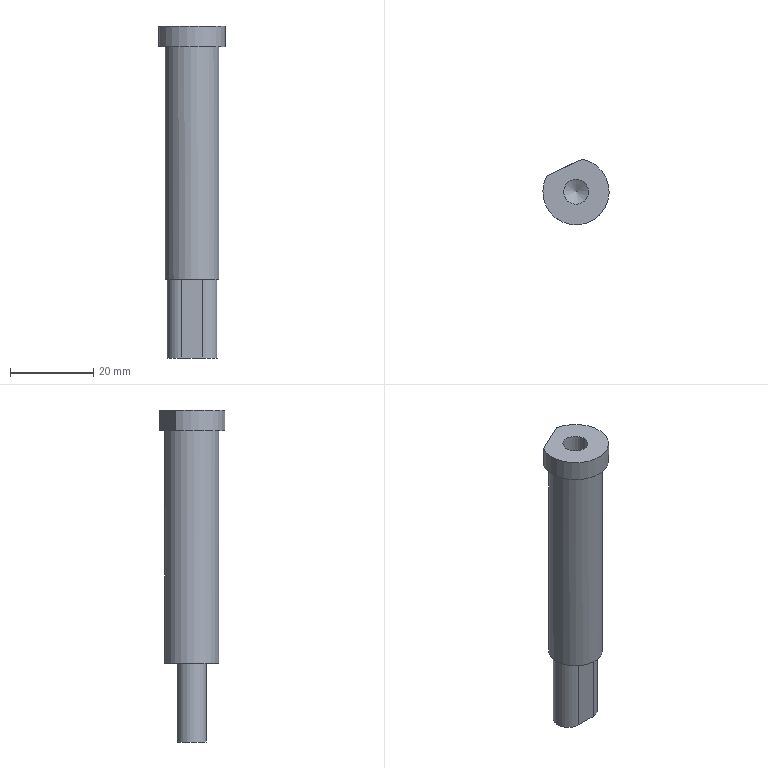Part | NX | features solid 2 | 1 solid | 13 faces | box 16 x 15.862 x 80 mm | volume 9434 mm3 | plane 7 | cylinder 5 | cone 1 | commonest cylinder face diameters 7.1 x2 6 x1 13 x1 16 x1
STEP:
#1=CARTESIAN_POINT('',(-654.921,-401.954,29.));
#2=VERTEX_POINT('',#1);
#3=CARTESIAN_POINT('',(-654.921,-408.454,29.));
#4=DIRECTION('',(0.,0.,1.));
#5=DIRECTION('',(0.,1.,0.));
#6=AXIS2_PLACEMENT_3D('',#3,#4,#5);
#7=CIRCLE('',#6,6.5);
#8=EDGE_CURVE('',#2,#2,#7,.T.);
#9=ORIENTED_EDGE('',*,*,#8,.F.);
#10=EDGE_LOOP('',(#9));
#11=FACE_BOUND('',#10,.T.);
#12=CARTESIAN_POINT('',(-657.421,-404.904,29.));
#13=VERTEX_POINT('',#12);
#14=CARTESIAN_POINT('',(-652.421,-404.904,29.));
#15=VERTEX_POINT('',#14);
#16=CARTESIAN_POINT('',(-654.921,-404.904,29.));
#17=DIRECTION('',(1.,0.,0.));
#18=VECTOR('',#17,1000.);
#19=LINE('',#16,#18);
#20=EDGE_CURVE('',#13,#15,#19,.T.);
#21=ORIENTED_EDGE('',*,*,#20,.F.);
#22=CARTESIAN_POINT('',(-657.421,-412.004,29.));
#23=VERTEX_POINT('',#22);
#24=CARTESIAN_POINT('',(-657.421,-408.454,29.));
#25=DIRECTION('',(0.,0.,1.));
#26=DIRECTION('',(0.,1.,0.));
#27=AXIS2_PLACEMENT_3D('',#24,#25,#26);
#28=CIRCLE('',#27,3.55);
#29=EDGE_CURVE('',#13,#23,#28,.T.);
#30=ORIENTED_EDGE('',*,*,#29,.T.);
#31=CARTESIAN_POINT('',(-652.421,-412.004,29.));
#32=VERTEX_POINT('',#31);
#33=CARTESIAN_POINT('',(-654.921,-412.004,29.));
#34=DIRECTION('',(1.,0.,0.));
#35=VECTOR('',#34,1000.);
#36=LINE('',#33,#35);
#37=EDGE_CURVE('',#23,#32,#36,.T.);
#38=ORIENTED_EDGE('',*,*,#37,.T.);
#39=CARTESIAN_POINT('',(-652.421,-408.454,29.));
#40=DIRECTION('',(0.,0.,1.));
#41=DIRECTION('',(0.,1.,0.));
#42=AXIS2_PLACEMENT_3D('',#39,#40,#41);
#43=CIRCLE('',#42,3.55);
#44=EDGE_CURVE('',#32,#15,#43,.T.);
#45=ORIENTED_EDGE('',*,*,#44,.T.);
#46=EDGE_LOOP('',(#21,#30,#38,#45));
#47=FACE_BOUND('',#46,.T.);
#48=CARTESIAN_POINT('',(-654.921,-408.454,29.));
#49=DIRECTION('',(0.,0.,1.));
#50=DIRECTION('',(0.,1.,0.));
#51=AXIS2_PLACEMENT_3D('',#48,#49,#50);
#52=PLANE('',#51);
#53=ADVANCED_FACE('',(#11,#47),#52,.F.);
#54=ORIENTED_EDGE('',*,*,#8,.T.);
#55=EDGE_LOOP('',(#54));
#56=FACE_BOUND('',#55,.T.);
#57=CARTESIAN_POINT('',(-657.668,-402.563,85.));
#58=VERTEX_POINT('',#57);
#59=CARTESIAN_POINT('',(-654.921,-408.454,85.));
#60=DIRECTION('',(0.,0.,1.));
#61=DIRECTION('',(0.,1.,0.));
#62=AXIS2_PLACEMENT_3D('',#59,#60,#61);
#63=CIRCLE('',#62,6.5);
#64=EDGE_CURVE('',#58,#58,#63,.T.);
#65=ORIENTED_EDGE('',*,*,#64,.F.);
#66=EDGE_LOOP('',(#65));
#67=FACE_BOUND('',#66,.T.);
#68=CARTESIAN_POINT('',(-654.921,-408.454,90.));
#69=DIRECTION('',(0.,0.,-1.));
#70=DIRECTION('',(0.,-1.,0.));
#71=AXIS2_PLACEMENT_3D('',#68,#69,#70);
#72=CYLINDRICAL_SURFACE('',#71,6.5);
#73=ADVANCED_FACE('',(#56,#67),#72,.T.);
#74=CARTESIAN_POINT('',(-661.894,-404.534,85.));
#75=VERTEX_POINT('',#74);
#76=CARTESIAN_POINT('',(-653.441,-400.592,85.));
#77=VERTEX_POINT('',#76);
#78=CARTESIAN_POINT('',(-654.921,-408.454,85.));
#79=DIRECTION('',(0.,0.,1.));
#80=DIRECTION('',(0.,1.,0.));
#81=AXIS2_PLACEMENT_3D('',#78,#79,#80);
#82=CIRCLE('',#81,8.);
#83=EDGE_CURVE('',#75,#77,#82,.T.);
#84=ORIENTED_EDGE('',*,*,#83,.F.);
#85=CARTESIAN_POINT('',(-653.441,-400.592,85.));
#86=DIRECTION('',(0.9063,0.4226,0.));
#87=VECTOR('',#86,1000.);
#88=LINE('',#85,#87);
#89=EDGE_CURVE('',#75,#58,#88,.T.);
#90=ORIENTED_EDGE('',*,*,#89,.T.);
#91=ORIENTED_EDGE('',*,*,#64,.T.);
#92=CARTESIAN_POINT('',(-653.441,-400.592,85.));
#93=DIRECTION('',(0.9063,0.4226,0.));
#94=VECTOR('',#93,1000.);
#95=LINE('',#92,#94);
#96=EDGE_CURVE('',#58,#77,#95,.T.);
#97=ORIENTED_EDGE('',*,*,#96,.T.);
#98=EDGE_LOOP('',(#84,#90,#91,#97));
#99=FACE_BOUND('',#98,.T.);
#100=CARTESIAN_POINT('',(-654.921,-408.454,85.));
#101=DIRECTION('',(0.,0.,1.));
#102=DIRECTION('',(0.,1.,0.));
#103=AXIS2_PLACEMENT_3D('',#100,#101,#102);
#104=PLANE('',#103);
#105=ADVANCED_FACE('',(#99),#104,.F.);
#106=CARTESIAN_POINT('',(-653.441,-400.592,90.));
#107=VERTEX_POINT('',#106);
#108=CARTESIAN_POINT('',(-653.441,-400.592,-87.));
#109=DIRECTION('',(0.,0.,-1.));
#110=VECTOR('',#109,1000.);
#111=LINE('',#108,#110);
#112=EDGE_CURVE('',#107,#77,#111,.T.);
#113=ORIENTED_EDGE('',*,*,#112,.F.);
#114=CARTESIAN_POINT('',(-661.894,-404.534,90.));
#115=VERTEX_POINT('',#114);
#116=CARTESIAN_POINT('',(-654.921,-408.454,90.));
#117=DIRECTION('',(0.,0.,1.));
#118=DIRECTION('',(0.,1.,0.));
#119=AXIS2_PLACEMENT_3D('',#116,#117,#118);
#120=CIRCLE('',#119,8.);
#121=EDGE_CURVE('',#115,#107,#120,.T.);
#122=ORIENTED_EDGE('',*,*,#121,.F.);
#123=CARTESIAN_POINT('',(-661.894,-404.534,-87.));
#124=DIRECTION('',(0.,0.,-1.));
#125=VECTOR('',#124,1000.);
#126=LINE('',#123,#125);
#127=EDGE_CURVE('',#75,#115,#126,.F.);
#128=ORIENTED_EDGE('',*,*,#127,.F.);
#129=ORIENTED_EDGE('',*,*,#83,.T.);
#130=EDGE_LOOP('',(#113,#122,#128,#129));
#131=FACE_BOUND('',#130,.T.);
#132=CARTESIAN_POINT('',(-654.921,-408.454,85.));
#133=DIRECTION('',(0.,0.,1.));
#134=DIRECTION('',(0.,1.,0.));
#135=AXIS2_PLACEMENT_3D('',#132,#133,#134);
#136=CYLINDRICAL_SURFACE('',#135,8.);
#137=ADVANCED_FACE('',(#131),#136,.T.);
#138=CARTESIAN_POINT('',(-654.921,-411.454,90.));
#139=VERTEX_POINT('',#138);
#140=CARTESIAN_POINT('',(-654.921,-408.454,90.));
#141=DIRECTION('',(0.,0.,-1.));
#142=DIRECTION('',(0.,-1.,0.));
#143=AXIS2_PLACEMENT_3D('',#140,#141,#142);
#144=CIRCLE('',#143,3.);
#145=EDGE_CURVE('',#139,#139,#144,.T.);
#146=ORIENTED_EDGE('',*,*,#145,.T.);
#147=EDGE_LOOP('',(#146));
#148=FACE_BOUND('',#147,.T.);
#149=CARTESIAN_POINT('',(-653.441,-400.592,90.));
#150=DIRECTION('',(0.9063,0.4226,0.));
#151=VECTOR('',#150,1000.);
#152=LINE('',#149,#151);
#153=EDGE_CURVE('',#115,#107,#152,.T.);
#154=ORIENTED_EDGE('',*,*,#153,.F.);
#155=ORIENTED_EDGE('',*,*,#121,.T.);
#156=EDGE_LOOP('',(#154,#155));
#157=FACE_BOUND('',#156,.T.);
#158=CARTESIAN_POINT('',(-654.921,-408.454,90.));
#159=DIRECTION('',(0.,0.,1.));
#160=DIRECTION('',(0.,1.,0.));
#161=AXIS2_PLACEMENT_3D('',#158,#159,#160);
#162=PLANE('',#161);
#163=ADVANCED_FACE('',(#148,#157),#162,.T.);
#164=ORIENTED_EDGE('',*,*,#127,.T.);
#165=ORIENTED_EDGE('',*,*,#153,.T.);
#166=ORIENTED_EDGE('',*,*,#112,.T.);
#167=ORIENTED_EDGE('',*,*,#96,.F.);
#168=ORIENTED_EDGE('',*,*,#89,.F.);
#169=EDGE_LOOP('',(#164,#165,#166,#167,#168));
#170=FACE_BOUND('',#169,.T.);
#171=CARTESIAN_POINT('',(-653.441,-400.592,-87.));
#172=DIRECTION('',(0.4226,-0.9063,0.));
#173=DIRECTION('',(0.,0.,-1.));
#174=AXIS2_PLACEMENT_3D('',#171,#172,#173);
#175=PLANE('',#174);
#176=ADVANCED_FACE('',(#170),#175,.F.);
#177=CARTESIAN_POINT('',(-657.421,-404.904,10.));
#178=VERTEX_POINT('',#177);
#179=CARTESIAN_POINT('',(-657.421,-404.904,10.));
#180=DIRECTION('',(0.,0.,1.));
#181=VECTOR('',#180,1000.);
#182=LINE('',#179,#181);
#183=EDGE_CURVE('',#178,#13,#182,.T.);
#184=ORIENTED_EDGE('',*,*,#183,.T.);
#185=ORIENTED_EDGE('',*,*,#20,.T.);
#186=CARTESIAN_POINT('',(-652.421,-404.904,10.));
#187=VERTEX_POINT('',#186);
#188=CARTESIAN_POINT('',(-652.421,-404.904,10.));
#189=DIRECTION('',(0.,0.,1.));
#190=VECTOR('',#189,1000.);
#191=LINE('',#188,#190);
#192=EDGE_CURVE('',#187,#15,#191,.T.);
#193=ORIENTED_EDGE('',*,*,#192,.F.);
#194=CARTESIAN_POINT('',(-657.421,-404.904,10.));
#195=DIRECTION('',(1.,0.,0.));
#196=VECTOR('',#195,1000.);
#197=LINE('',#194,#196);
#198=EDGE_CURVE('',#178,#187,#197,.T.);
#199=ORIENTED_EDGE('',*,*,#198,.F.);
#200=EDGE_LOOP('',(#184,#185,#193,#199));
#201=FACE_BOUND('',#200,.T.);
#202=CARTESIAN_POINT('',(-657.421,-404.904,10.));
#203=DIRECTION('',(0.,-1.,0.));
#204=DIRECTION('',(0.,0.,1.));
#205=AXIS2_PLACEMENT_3D('',#202,#203,#204);
#206=PLANE('',#205);
#207=ADVANCED_FACE('',(#201),#206,.F.);
#208=ORIENTED_EDGE('',*,*,#44,.F.);
#209=CARTESIAN_POINT('',(-652.421,-412.004,10.));
#210=VERTEX_POINT('',#209);
#211=CARTESIAN_POINT('',(-652.421,-412.004,10.));
#212=DIRECTION('',(0.,0.,1.));
#213=VECTOR('',#212,1000.);
#214=LINE('',#211,#213);
#215=EDGE_CURVE('',#210,#32,#214,.T.);
#216=ORIENTED_EDGE('',*,*,#215,.F.);
#217=CARTESIAN_POINT('',(-652.421,-408.454,10.));
#218=DIRECTION('',(0.,0.,1.));
#219=DIRECTION('',(0.,1.,0.));
#220=AXIS2_PLACEMENT_3D('',#217,#218,#219);
#221=CIRCLE('',#220,3.55);
#222=EDGE_CURVE('',#210,#187,#221,.T.);
#223=ORIENTED_EDGE('',*,*,#222,.T.);
#224=ORIENTED_EDGE('',*,*,#192,.T.);
#225=EDGE_LOOP('',(#208,#216,#223,#224));
#226=FACE_BOUND('',#225,.T.);
#227=CARTESIAN_POINT('',(-652.421,-408.454,10.));
#228=DIRECTION('',(0.,0.,1.));
#229=DIRECTION('',(0.,1.,0.));
#230=AXIS2_PLACEMENT_3D('',#227,#228,#229);
#231=CYLINDRICAL_SURFACE('',#230,3.55);
#232=ADVANCED_FACE('',(#226),#231,.T.);
#233=ORIENTED_EDGE('',*,*,#37,.F.);
#234=CARTESIAN_POINT('',(-657.421,-412.004,10.));
#235=VERTEX_POINT('',#234);
#236=CARTESIAN_POINT('',(-657.421,-412.004,10.));
#237=DIRECTION('',(0.,0.,1.));
#238=VECTOR('',#237,1000.);
#239=LINE('',#236,#238);
#240=EDGE_CURVE('',#235,#23,#239,.T.);
#241=ORIENTED_EDGE('',*,*,#240,.F.);
#242=CARTESIAN_POINT('',(-657.421,-412.004,10.));
#243=DIRECTION('',(1.,0.,0.));
#244=VECTOR('',#243,1000.);
#245=LINE('',#242,#244);
#246=EDGE_CURVE('',#235,#210,#245,.T.);
#247=ORIENTED_EDGE('',*,*,#246,.T.);
#248=ORIENTED_EDGE('',*,*,#215,.T.);
#249=EDGE_LOOP('',(#233,#241,#247,#248));
#250=FACE_BOUND('',#249,.T.);
#251=CARTESIAN_POINT('',(-657.421,-412.004,10.));
#252=DIRECTION('',(0.,-1.,0.));
#253=DIRECTION('',(0.,0.,1.));
#254=AXIS2_PLACEMENT_3D('',#251,#252,#253);
#255=PLANE('',#254);
#256=ADVANCED_FACE('',(#250),#255,.T.);
#257=ORIENTED_EDGE('',*,*,#29,.F.);
#258=ORIENTED_EDGE('',*,*,#183,.F.);
#259=CARTESIAN_POINT('',(-657.421,-408.454,10.));
#260=DIRECTION('',(0.,0.,1.));
#261=DIRECTION('',(0.,1.,0.));
#262=AXIS2_PLACEMENT_3D('',#259,#260,#261);
#263=CIRCLE('',#262,3.55);
#264=EDGE_CURVE('',#178,#235,#263,.T.);
#265=ORIENTED_EDGE('',*,*,#264,.T.);
#266=ORIENTED_EDGE('',*,*,#240,.T.);
#267=EDGE_LOOP('',(#257,#258,#265,#266));
#268=FACE_BOUND('',#267,.T.);
#269=CARTESIAN_POINT('',(-657.421,-408.454,10.));
#270=DIRECTION('',(0.,0.,1.));
#271=DIRECTION('',(0.,1.,0.));
#272=AXIS2_PLACEMENT_3D('',#269,#270,#271);
#273=CYLINDRICAL_SURFACE('',#272,3.55);
#274=ADVANCED_FACE('',(#268),#273,.T.);
#275=ORIENTED_EDGE('',*,*,#198,.T.);
#276=ORIENTED_EDGE('',*,*,#222,.F.);
#277=ORIENTED_EDGE('',*,*,#246,.F.);
#278=ORIENTED_EDGE('',*,*,#264,.F.);
#279=EDGE_LOOP('',(#275,#276,#277,#278));
#280=FACE_BOUND('',#279,.T.);
#281=CARTESIAN_POINT('',(-652.421,-408.454,10.));
#282=DIRECTION('',(0.,0.,1.));
#283=DIRECTION('',(0.,1.,0.));
#284=AXIS2_PLACEMENT_3D('',#281,#282,#283);
#285=PLANE('',#284);
#286=ADVANCED_FACE('',(#280),#285,.F.);
#287=CARTESIAN_POINT('',(-654.921,-411.454,77.));
#288=VERTEX_POINT('',#287);
#289=CARTESIAN_POINT('',(-654.921,-408.454,77.));
#290=DIRECTION('',(0.,0.,-1.));
#291=DIRECTION('',(0.,-1.,0.));
#292=AXIS2_PLACEMENT_3D('',#289,#290,#291);
#293=CIRCLE('',#292,3.);
#294=EDGE_CURVE('',#288,#288,#293,.T.);
#295=ORIENTED_EDGE('',*,*,#294,.F.);
#296=EDGE_LOOP('',(#295));
#297=FACE_BOUND('',#296,.T.);
#298=CARTESIAN_POINT('',(-654.921,-408.454,75.268));
#299=VERTEX_POINT('',#298);
#300=VERTEX_LOOP('',#299);
#301=FACE_BOUND('',#300,.T.);
#302=CARTESIAN_POINT('',(-654.921,-408.454,77.));
#303=DIRECTION('',(0.,0.,1.));
#304=DIRECTION('',(0.,1.,0.));
#305=AXIS2_PLACEMENT_3D('',#302,#303,#304);
#306=CONICAL_SURFACE('',#305,3.,1.047);
#307=ADVANCED_FACE('',(#297,#301),#306,.F.);
#308=ORIENTED_EDGE('',*,*,#294,.T.);
#309=EDGE_LOOP('',(#308));
#310=FACE_BOUND('',#309,.T.);
#311=ORIENTED_EDGE('',*,*,#145,.F.);
#312=EDGE_LOOP('',(#311));
#313=FACE_BOUND('',#312,.T.);
#314=CARTESIAN_POINT('',(-654.921,-408.454,90.));
#315=DIRECTION('',(0.,0.,-1.));
#316=DIRECTION('',(0.,-1.,0.));
#317=AXIS2_PLACEMENT_3D('',#314,#315,#316);
#318=CYLINDRICAL_SURFACE('',#317,3.);
#319=ADVANCED_FACE('',(#310,#313),#318,.F.);
#320=CLOSED_SHELL('',(#53,#73,#105,#137,#163,#176,#207,#232,#256,#274,#286,#307,#319));
#321=MANIFOLD_SOLID_BREP('',#320);
#322=(LENGTH_UNIT()NAMED_UNIT(*)SI_UNIT(.MILLI.,.METRE.));
#323=UNCERTAINTY_MEASURE_WITH_UNIT(LENGTH_MEASURE(0.00001),#322,'','');
#324=(NAMED_UNIT(*)PLANE_ANGLE_UNIT()SI_UNIT($,.RADIAN.));
#325=(NAMED_UNIT(*)SI_UNIT($,.STERADIAN.)SOLID_ANGLE_UNIT());
#326=(GEOMETRIC_REPRESENTATION_CONTEXT(3)GLOBAL_UNCERTAINTY_ASSIGNED_CONTEXT((#323))GLOBAL_UNIT_ASSIGNED_CONTEXT((#322,#324,#325))REPRESENTATION_CONTEXT('',''));
#327=ADVANCED_BREP_SHAPE_REPRESENTATION('',(#321),#326);